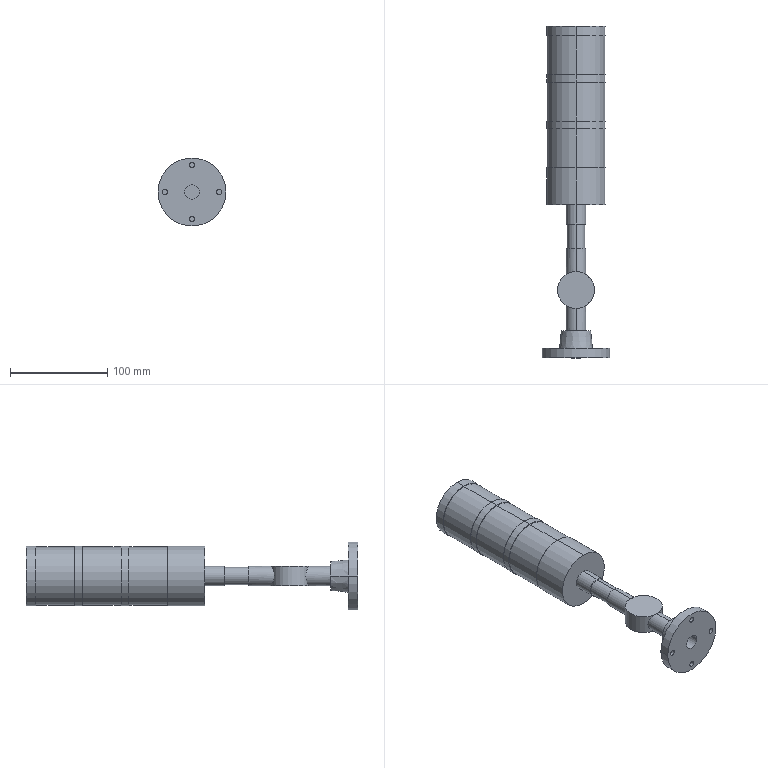Part | STEP file | foldable alarm light | 1 solid | 55 faces | box 70 x 342 x 70 mm | volume 623933 mm3 | cylinder 37 | plane 16 | cone 2 | commonest cylinder face diameters 5.5 x8 61 x8 20 x6 60 x6 38 x3 15 x2